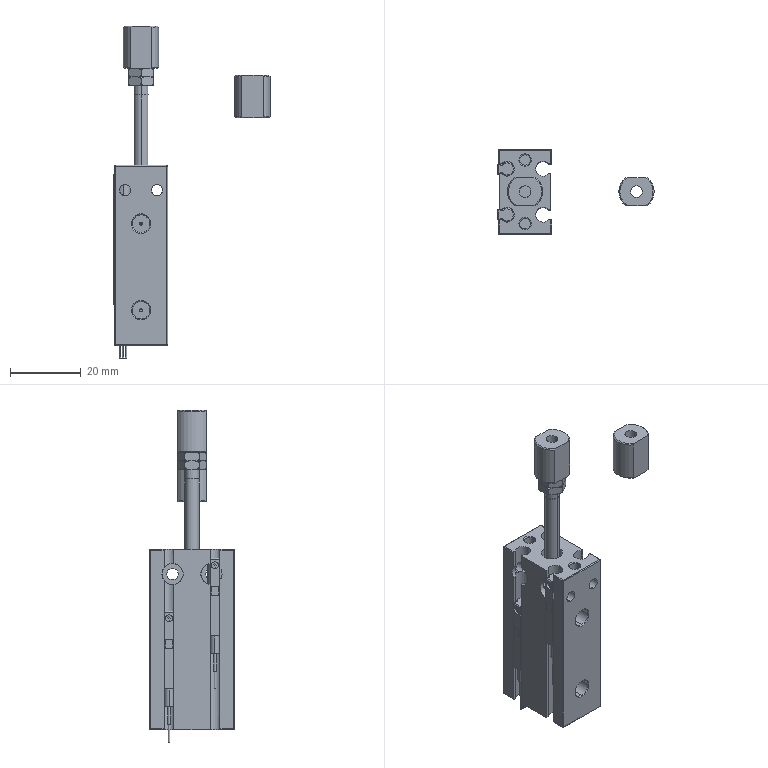Part | NX | 7 solids | 327 faces | box 44.21 x 24 x 93.9 mm | volume 15311 mm3 | cylinder 146 | plane 111 | cone 36 | torus 22 | sphere 8 | spline 4 | commonest cylinder face diameters 0.5 x28 3.2 x16 4 x14 6 x14 0.75 x12 4.2 x12